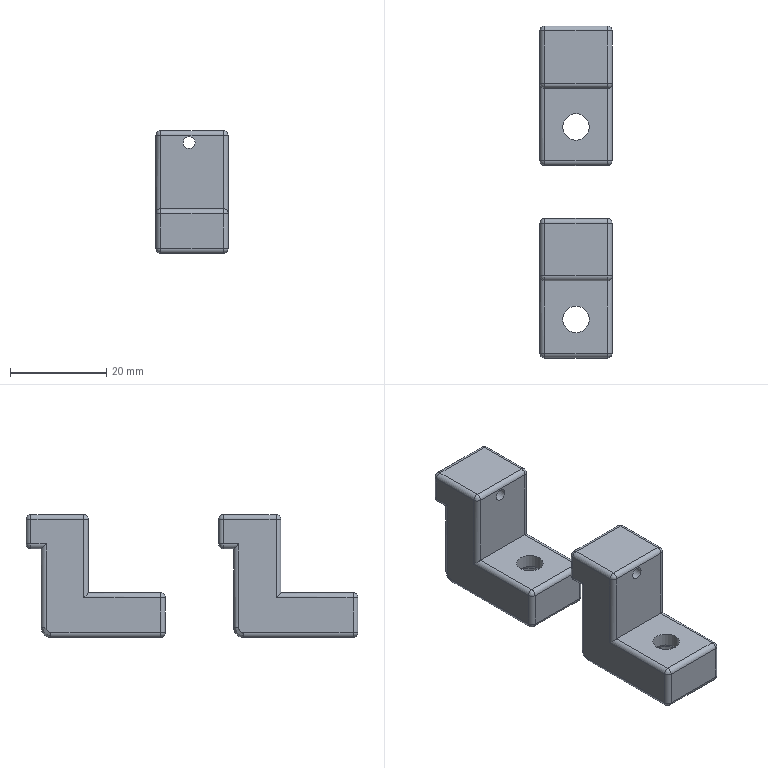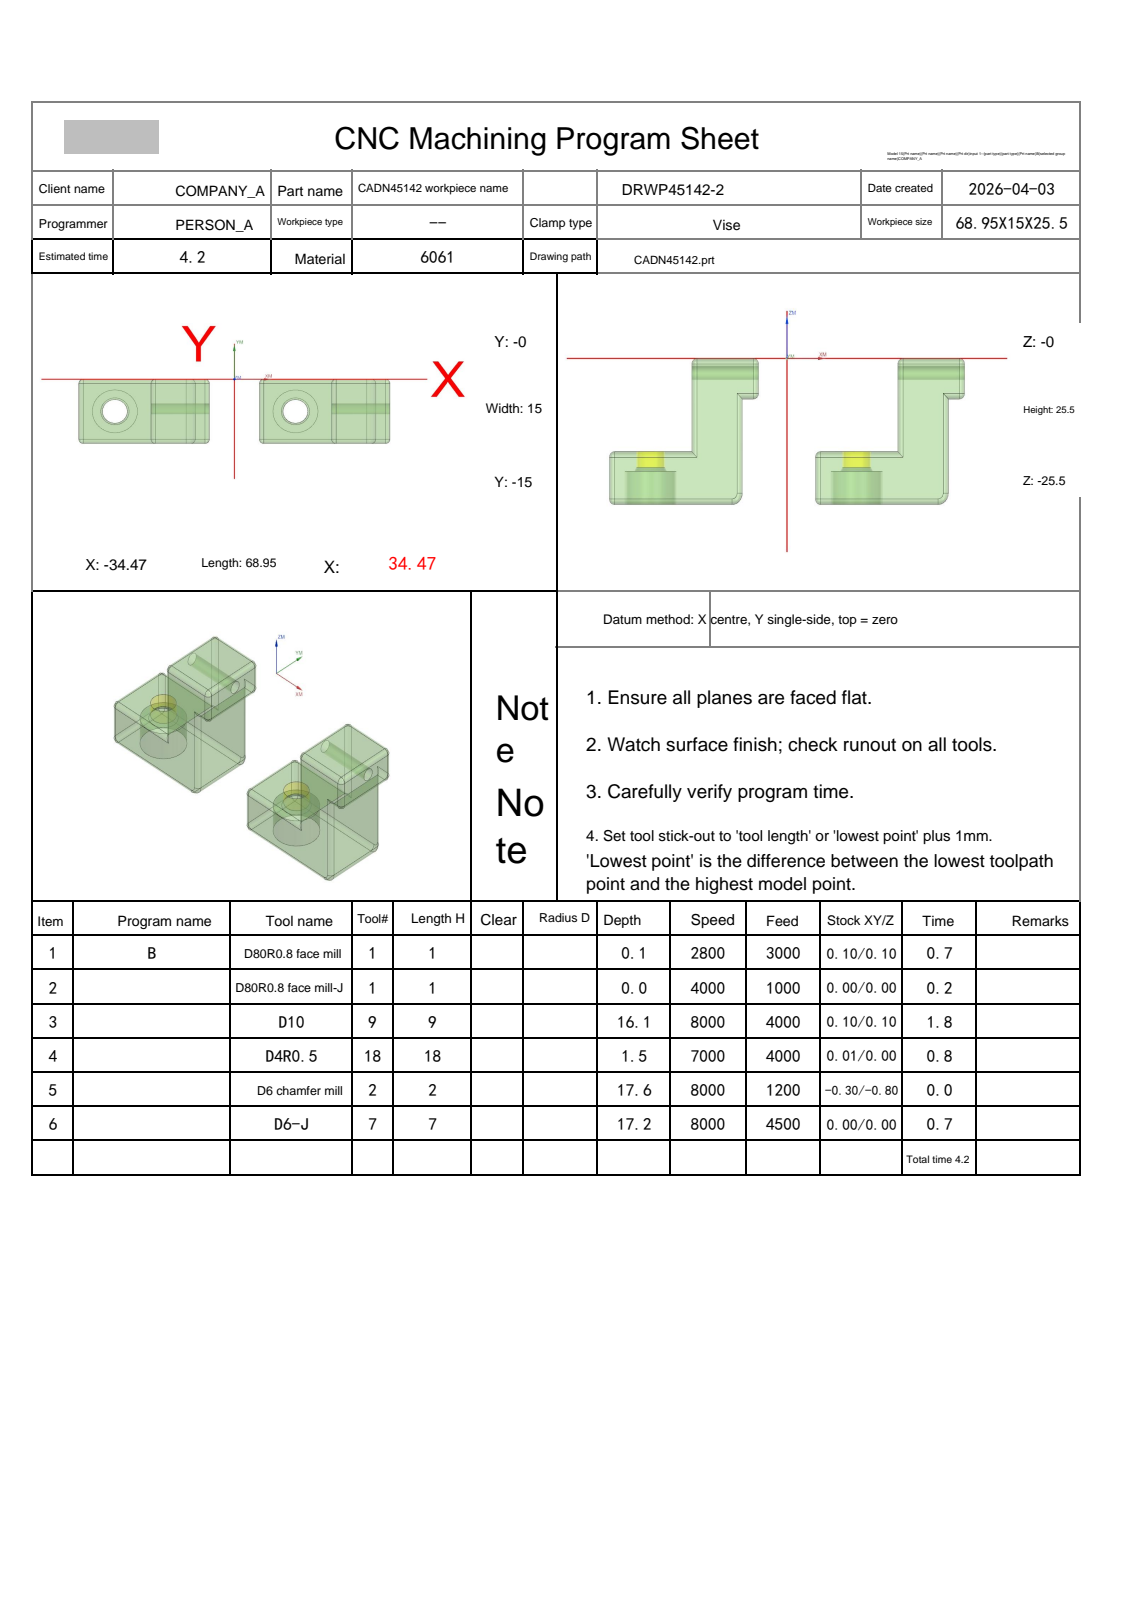NC program | NX | posted by the shop | part box 15 x 68.95 x 25.5 mm
Lines 1 to 1497 of 8513:
%
O0001
(Machine time: 5.39 MIN)
(===Total Tool:5===)
(T1=D80R0.8 face mill D=80.  R=0.8  D-  H01 Z=-0.   )
(T9=D10     D=10.  R=0.   D-  H09 Z=-16.15)
(T18=D4R0.5 D=4.   R=0.5  D-  H18 Z=-1.5  )
(T2=D6 chamfer mill   D=6.   R=0.   D-  H02 Z=-17.65)
(T7=D6-J    D=6.   R=0.   D7  H07 Z=-17.25)
G80 G90 G17 G49 G40
G91 G28 Z0
M01
N1 T01 M06
(D80R0.8 face mill D=80. R=0.8 H=01 ce=0.10 di=0.10)
G00 G90 G54 X86.572 Y-5.569 M03 S2800
G43 H01 Z20.
M08
Z6.011
G01 Z4.011 F3000.
X74.572 Y-5.836
X-74.572 Y-9.163
X-86.572 Y-9.431
Z6.011
G00 X86.572 Y-5.569
Z5.522
G01 Z3.522
X74.572 Y-5.836
X-74.572 Y-9.163
X-86.572 Y-9.431
Z5.522
G00 X86.572 Y-5.569
Z5.033
G01 Z3.033
X74.572 Y-5.836
X-74.572 Y-9.163
X-86.572 Y-9.431
Z5.033
G00 X86.572 Y-5.569
Z4.544
G01 Z2.544
X74.572 Y-5.836
X-74.572 Y-9.163
X-86.572 Y-9.431
Z4.544
G00 Z20.
X86.572 Y-5.569
Z4.056
G01 Z2.056
X74.572 Y-5.836
X-74.572 Y-9.163
X-86.572 Y-9.431
Z4.056
G00 Z20.
X86.572 Y-5.569
Z3.567
G01 Z1.567
X74.572 Y-5.836
X-74.572 Y-9.163
X-86.572 Y-9.431
Z3.567
G00 Z20.
X86.572 Y-5.569
Z3.078
G01 Z1.078
X74.572 Y-5.836
X-74.572 Y-9.163
X-86.572 Y-9.431
Z3.078
G00 Z20.
X86.572 Y-5.569
Z2.589
G01 Z.589
X74.572 Y-5.836
X-74.572 Y-9.163
X-86.572 Y-9.431
Z2.589
G00 Z20.
X86.572 Y-5.569
Z2.1
G01 Z.1
X74.572 Y-5.836
X-74.572 Y-9.163
X-86.572 Y-9.431
Z2.1
G00 Z20.
G91 G28 Z0.0
M05
M09
G91 G28 Z0.0
M01
N2 T01 M06
(D80R0.8 face mill-J  D=80. R=0.8 H=01 ce=0.00 di=0.00)
G00 G90 G54 X86.474 Y-5.572 M03 S4000
G43 H01 Z20.
M08
Z2.
G01 Z0.0 F1000.
X74.474 Y-5.84
X-74.474 Y-9.16
X-86.474 Y-9.427
Z2.
G00 Z20.
G91 G28 Z0.0
M05
M09
G91 G28 Z0.0
M01
N3 T09 M06
(D10  D=10. R=0. H=09 ce=0.10 di=0.10)
G00 G90 G54 X9.025 Y7. M03 S8000
G43 H09 Z14.
M08
Z.902
G01 Z-.598 F4000.
Y3.9
X18.892
G03 X16.425 Y-1. I3.633 J-4.9
G01 Y-14.
G03 X18.892 Y-18.9 I6.1 J0.0
G01 X1.625
Y3.9
X6.357
G02 X7.069 Y3.602 I0.0 J-1.
G01 X11.138 Y-.529
G03 X11.388 Y-.713 I.712 J.702
G02 X11.925 Y-1.599 I-.462 J-.887
G01 Y-13.401
G02 X10.927 Y-14.4 I-1. J.001
G01 X7.124
G02 X6.125 Y-13.401 I.001 J1.
G01 Y-1.599
G02 X7.124 Y-.6 I1. J-.001
G01 X9.025
X9.525
Y7.
Z.902
G00 X9.025
Z.304
G01 Z-1.196
Y3.9
X18.892
G03 X16.425 Y-1. I3.633 J-4.9
G01 Y-14.
G03 X18.892 Y-18.9 I6.1 J0.0
G01 X1.625
Y3.9
X6.357
G02 X7.069 Y3.602 I0.0 J-1.
G01 X11.138 Y-.529
G03 X11.388 Y-.713 I.712 J.702
G02 X11.925 Y-1.599 I-.462 J-.887
G01 Y-13.401
G02 X10.927 Y-14.4 I-1. J.001
G01 X7.124
G02 X6.125 Y-13.401 I.001 J1.
G01 Y-1.599
G02 X7.124 Y-.6 I1. J-.001
G01 X9.025
X9.525
Y7.
Z.304
G00 X9.025
Z-.294
G01 Z-1.794
Y3.9
X18.892
G03 X16.425 Y-1. I3.633 J-4.9
G01 Y-14.
G03 X18.892 Y-18.9 I6.1 J0.0
G01 X1.625
Y3.9
X6.357
G02 X7.069 Y3.602 I0.0 J-1.
G01 X11.138 Y-.529
G03 X11.388 Y-.713 I.712 J.702
G02 X11.925 Y-1.599 I-.462 J-.887
G01 Y-13.401
G02 X10.927 Y-14.4 I-1. J.001
G01 X7.124
G02 X6.125 Y-13.401 I.001 J1.
G01 Y-1.599
G02 X7.124 Y-.6 I1. J-.001
G01 X9.025
X9.525
Y7.
Z-.294
G00 X9.025
Z-.893
G01 Z-2.393
Y3.9
X18.892
G03 X16.425 Y-1. I3.633 J-4.9
G01 Y-14.
G03 X18.892 Y-18.9 I6.1 J0.0
G01 X1.625
Y3.9
X6.357
G02 X7.069 Y3.602 I0.0 J-1.
G01 X11.138 Y-.529
G03 X11.388 Y-.713 I.712 J.702
G02 X11.925 Y-1.599 I-.462 J-.887
G01 Y-13.401
G02 X10.927 Y-14.4 I-1. J.001
G01 X7.124
G02 X6.125 Y-13.401 I.001 J1.
G01 Y-1.599
G02 X7.124 Y-.6 I1. J-.001
G01 X9.025
X9.525
Y7.
Z-.893
G00 X9.025
Z-1.491
G01 Z-2.991
Y3.9
X18.892
G03 X16.425 Y-1. I3.633 J-4.9
G01 Y-14.
G03 X18.892 Y-18.9 I6.1 J0.0
G01 X1.625
Y3.9
X6.357
G02 X7.069 Y3.602 I0.0 J-1.
G01 X11.138 Y-.529
G03 X11.388 Y-.713 I.712 J.702
G02 X11.925 Y-1.599 I-.462 J-.887
G01 Y-13.401
G02 X10.927 Y-14.4 I-1. J.001
G01 X7.124
G02 X6.125 Y-13.401 I.001 J1.
G01 Y-1.599
G02 X7.124 Y-.6 I1. J-.001
G01 X9.025
X9.525
Y7.
Z-1.491
G00 X9.025
Z-2.089
G01 Z-3.589
Y3.9
X18.892
G03 X16.425 Y-1. I3.633 J-4.9
G01 Y-14.
G03 X18.892 Y-18.9 I6.1 J0.0
G01 X1.625
Y3.9
X6.357
G02 X7.069 Y3.602 I0.0 J-1.
G01 X11.138 Y-.529
G03 X11.388 Y-.713 I.712 J.702
G02 X11.925 Y-1.599 I-.462 J-.887
G01 Y-13.401
G02 X10.927 Y-14.4 I-1. J.001
G01 X7.124
G02 X6.125 Y-13.401 I.001 J1.
G01 Y-1.599
G02 X7.124 Y-.6 I1. J-.001
G01 X9.025
X9.525
Y7.
Z-2.089
G00 X9.025
Z-2.687
G01 Z-4.187
Y3.9
X18.892
G03 X16.425 Y-1. I3.633 J-4.9
G01 Y-14.
G03 X18.892 Y-18.9 I6.1 J0.0
G01 X1.625
Y3.9
X6.357
G02 X7.069 Y3.602 I0.0 J-1.
G01 X11.138 Y-.529
G03 X11.388 Y-.713 I.712 J.702
G02 X11.925 Y-1.599 I-.462 J-.887
G01 Y-13.401
G02 X10.927 Y-14.4 I-1. J.001
G01 X7.124
G02 X6.125 Y-13.401 I.001 J1.
G01 Y-1.599
G02 X7.124 Y-.6 I1. J-.001
G01 X9.025
X9.525
Y7.
Z-2.687
G00 X9.025
Z-3.285
G01 Z-4.785
Y3.9
X18.892
G03 X16.425 Y-1. I3.633 J-4.9
G01 Y-14.
G03 X18.892 Y-18.9 I6.1 J0.0
G01 X1.625
Y3.9
X6.357
G02 X7.069 Y3.602 I0.0 J-1.
G01 X11.138 Y-.529
G03 X11.388 Y-.713 I.712 J.702
G02 X11.925 Y-1.599 I-.462 J-.887
G01 Y-13.401
G02 X10.927 Y-14.4 I-1. J.001
G01 X7.124
G02 X6.125 Y-13.401 I.001 J1.
G01 Y-1.599
G02 X7.124 Y-.6 I1. J-.001
G01 X9.025
X9.525
Y7.
Z-3.285
G00 X9.025
Z-3.883
G01 Z-5.383
Y3.9
X18.892
G03 X16.425 Y-1. I3.633 J-4.9
G01 Y-14.
G03 X18.892 Y-18.9 I6.1 J0.0
G01 X1.625
Y3.9
X6.357
G02 X7.069 Y3.602 I0.0 J-1.
G01 X11.138 Y-.529
G03 X11.388 Y-.713 I.712 J.702
G02 X11.925 Y-1.599 I-.462 J-.887
G01 Y-13.401
G02 X10.927 Y-14.4 I-1. J.001
G01 X7.124
G02 X6.125 Y-13.401 I.001 J1.
G01 Y-1.599
G02 X7.124 Y-.6 I1. J-.001
G01 X9.025
X9.525
Y7.
Z-3.883
G00 X9.025
Z-4.481
G01 Z-5.981
Y3.9
X18.892
G03 X16.425 Y-1. I3.633 J-4.9
G01 Y-14.
G03 X18.892 Y-18.9 I6.1 J0.0
G01 X1.625
Y3.9
X6.357
G02 X7.069 Y3.602 I0.0 J-1.
G01 X11.138 Y-.529
G03 X11.388 Y-.713 I.712 J.702
G02 X11.925 Y-1.599 I-.462 J-.887
G01 Y-13.401
G02 X10.927 Y-14.4 I-1. J.001
G01 X7.124
G02 X6.125 Y-13.401 I.001 J1.
G01 Y-1.599
G02 X7.124 Y-.6 I1. J-.001
G01 X9.025
X9.525
Y7.
Z-4.481
G00 X9.025
Z-5.08
G01 Z-6.58
Y3.9
X18.892
G03 X16.425 Y-1. I3.633 J-4.9
G01 Y-14.
G03 X18.892 Y-18.9 I6.1 J0.0
G01 X1.625
Y3.9
X6.357
G02 X7.069 Y3.602 I0.0 J-1.
G01 X11.138 Y-.529
G03 X11.388 Y-.713 I.712 J.702
G02 X11.925 Y-1.599 I-.462 J-.887
G01 Y-13.401
G02 X10.927 Y-14.4 I-1. J.001
G01 X7.124
G02 X6.125 Y-13.401 I.001 J1.
G01 Y-1.599
G02 X7.124 Y-.6 I1. J-.001
G01 X9.025
X9.525
Y7.
Z-5.08
G00 X9.025
Z-5.678
G01 Z-7.178
Y3.9
X18.892
G03 X16.425 Y-1. I3.633 J-4.9
G01 Y-14.
G03 X18.892 Y-18.9 I6.1 J0.0
G01 X1.625
Y3.9
X6.357
G02 X7.069 Y3.602 I0.0 J-1.
G01 X11.138 Y-.529
G03 X11.388 Y-.713 I.712 J.702
G02 X11.925 Y-1.599 I-.462 J-.887
G01 Y-13.401
G02 X10.927 Y-14.4 I-1. J.001
G01 X7.124
G02 X6.125 Y-13.401 I.001 J1.
G01 Y-1.599
G02 X7.124 Y-.6 I1. J-.001
G01 X9.025
X9.525
Y7.
Z-5.678
G00 X9.025
Z-6.276
G01 Z-7.776
Y3.9
X18.892
G03 X16.425 Y-1. I3.633 J-4.9
G01 Y-14.
G03 X18.892 Y-18.9 I6.1 J0.0
G01 X1.625
Y3.9
X6.357
G02 X7.069 Y3.602 I0.0 J-1.
G01 X11.138 Y-.529
G03 X11.388 Y-.713 I.712 J.702
G02 X11.925 Y-1.599 I-.462 J-.887
G01 Y-13.401
G02 X10.927 Y-14.4 I-1. J.001
G01 X7.124
G02 X6.125 Y-13.401 I.001 J1.
G01 Y-1.599
G02 X7.124 Y-.6 I1. J-.001
G01 X9.025
X9.525
Y7.
Z-6.276
G00 X9.025
Z-6.874
G01 Z-8.374
Y3.9
X18.892
G03 X16.425 Y-1. I3.633 J-4.9
G01 Y-14.
G03 X18.892 Y-18.9 I6.1 J0.0
G01 X1.625
Y3.9
X6.357
G02 X7.069 Y3.602 I0.0 J-1.
G01 X11.138 Y-.529
G03 X11.388 Y-.713 I.712 J.702
G02 X11.925 Y-1.599 I-.462 J-.887
G01 Y-13.401
G02 X10.927 Y-14.4 I-1. J.001
G01 X7.124
G02 X6.125 Y-13.401 I.001 J1.
G01 Y-1.599
G02 X7.124 Y-.6 I1. J-.001
G01 X9.025
X9.525
Y7.
Z-6.874
G00 X9.025
Z-7.472
G01 Z-8.972
Y3.9
X18.892
G03 X16.425 Y-1. I3.633 J-4.9
G01 Y-14.
G03 X18.892 Y-18.9 I6.1 J0.0
G01 X1.625
Y3.9
X6.357
G02 X7.069 Y3.602 I0.0 J-1.
G01 X11.138 Y-.529
G03 X11.388 Y-.713 I.712 J.702
G02 X11.925 Y-1.599 I-.462 J-.887
G01 Y-13.401
G02 X10.927 Y-14.4 I-1. J.001
G01 X7.124
G02 X6.125 Y-13.401 I.001 J1.
G01 Y-1.599
G02 X7.124 Y-.6 I1. J-.001
G01 X9.025
X9.525
Y7.
Z-7.472
G00 X9.025
Z-8.07
G01 Z-9.57
Y3.9
X18.892
G03 X16.425 Y-1. I3.633 J-4.9
G01 Y-14.
G03 X18.892 Y-18.9 I6.1 J0.0
G01 X1.625
Y3.9
X6.357
G02 X7.069 Y3.602 I0.0 J-1.
G01 X11.138 Y-.529
G03 X11.388 Y-.713 I.712 J.702
G02 X11.925 Y-1.599 I-.462 J-.887
G01 Y-13.401
G02 X10.927 Y-14.4 I-1. J.001
G01 X7.124
G02 X6.125 Y-13.401 I.001 J1.
G01 Y-1.599
G02 X7.124 Y-.6 I1. J-.001
G01 X9.025
X9.525
Y7.
Z-8.07
G00 X9.025
Z-8.669
G01 Z-10.169
Y3.9
X18.892
G03 X16.425 Y-1. I3.633 J-4.9
G01 Y-14.
G03 X18.892 Y-18.9 I6.1 J0.0
G01 X1.625
Y3.9
X6.357
G02 X7.069 Y3.602 I0.0 J-1.
G01 X11.138 Y-.529
G03 X11.388 Y-.713 I.712 J.702
G02 X11.925 Y-1.599 I-.462 J-.887
G01 Y-13.401
G02 X10.927 Y-14.4 I-1. J.001
G01 X7.124
G02 X6.125 Y-13.401 I.001 J1.
G01 Y-1.599
G02 X7.124 Y-.6 I1. J-.001
G01 X9.025
X9.525
Y7.
Z-8.669
G00 X9.025
Z-9.267
G01 Z-10.767
Y3.9
X18.892
G03 X16.425 Y-1. I3.633 J-4.9
G01 Y-14.
G03 X18.892 Y-18.9 I6.1 J0.0
G01 X1.625
Y3.9
X6.357
G02 X7.069 Y3.602 I0.0 J-1.
G01 X11.138 Y-.529
G03 X11.388 Y-.713 I.712 J.702
G02 X11.925 Y-1.599 I-.462 J-.887
G01 Y-13.401
G02 X10.927 Y-14.4 I-1. J.001
G01 X7.124
G02 X6.125 Y-13.401 I.001 J1.
G01 Y-1.599
G02 X7.124 Y-.6 I1. J-.001
G01 X9.025
X9.525
Y7.
Z-9.267
G00 X9.025
Z-9.865
G01 Z-11.365
Y3.9
X18.892
G03 X16.425 Y-1. I3.633 J-4.9
G01 Y-14.
G03 X18.892 Y-18.9 I6.1 J0.0
G01 X1.625
Y3.9
X6.357
G02 X7.069 Y3.602 I0.0 J-1.
G01 X11.138 Y-.529
G03 X11.388 Y-.713 I.712 J.702
G02 X11.925 Y-1.599 I-.462 J-.887
G01 Y-13.401
G02 X10.927 Y-14.4 I-1. J.001
G01 X7.124
G02 X6.125 Y-13.401 I.001 J1.
G01 Y-1.599
G02 X7.124 Y-.6 I1. J-.001
G01 X9.025
X9.525
Y7.
Z-9.865
G00 X9.025
Z-10.463
G01 Z-11.963
Y3.9
X18.892
G03 X16.425 Y-1. I3.633 J-4.9
G01 Y-14.
G03 X18.892 Y-18.9 I6.1 J0.0
G01 X1.625
Y3.9
X6.357
G02 X7.069 Y3.602 I0.0 J-1.
G01 X11.138 Y-.529
G03 X11.388 Y-.713 I.712 J.702
G02 X11.925 Y-1.599 I-.462 J-.887
G01 Y-13.401
G02 X10.927 Y-14.4 I-1. J.001
G01 X7.124
G02 X6.125 Y-13.401 I.001 J1.
G01 Y-1.599
G02 X7.124 Y-.6 I1. J-.001
G01 X9.025
X9.525
Y7.
Z-10.463
G00 X9.025
Z-11.061
G01 Z-12.561
Y3.9
X18.892
G03 X16.425 Y-1. I3.633 J-4.9
G01 Y-14.
G03 X18.892 Y-18.9 I6.1 J0.0
G01 X1.625
Y3.9
X6.357
G02 X7.069 Y3.602 I0.0 J-1.
G01 X11.138 Y-.529
G03 X11.388 Y-.713 I.712 J.702
G02 X11.925 Y-1.599 I-.462 J-.887
G01 Y-13.401
G02 X10.927 Y-14.4 I-1. J.001
G01 X7.124
G02 X6.125 Y-13.401 I.001 J1.
G01 Y-1.599
G02 X7.124 Y-.6 I1. J-.001
G01 X9.025
X9.525
Y7.
Z-11.061
G00 X9.025
Z-11.659
G01 Z-13.159
Y3.9
X18.892
G03 X16.425 Y-1. I3.633 J-4.9
G01 Y-14.
G03 X18.892 Y-18.9 I6.1 J0.0
G01 X1.625
Y3.9
X6.357
G02 X7.069 Y3.602 I0.0 J-1.
G01 X11.138 Y-.529
G03 X11.388 Y-.713 I.712 J.702
G02 X11.925 Y-1.599 I-.462 J-.887
G01 Y-13.401
G02 X10.927 Y-14.4 I-1. J.001
G01 X7.124
G02 X6.125 Y-13.401 I.001 J1.
G01 Y-1.599
G02 X7.124 Y-.6 I1. J-.001
G01 X9.025
X9.525
Y7.
Z-11.659
G00 X9.025
Z-12.257
G01 Z-13.757
Y3.9
X18.892
G03 X16.425 Y-1. I3.633 J-4.9
G01 Y-14.
G03 X18.892 Y-18.9 I6.1 J0.0
G01 X1.625
Y3.9
X6.357
G02 X7.069 Y3.602 I0.0 J-1.
G01 X11.138 Y-.529
G03 X11.388 Y-.713 I.712 J.702
G02 X11.925 Y-1.599 I-.462 J-.887
G01 Y-13.401
G02 X10.927 Y-14.4 I-1. J.001
G01 X7.124
G02 X6.125 Y-13.401 I.001 J1.
G01 Y-1.599
G02 X7.124 Y-.6 I1. J-.001
G01 X9.025
X9.525
Y7.
Z-12.257
G00 X9.025
Z-12.856
G01 Z-14.356
Y3.9
X18.892
G03 X16.425 Y-1. I3.633 J-4.9
G01 Y-14.
G03 X18.892 Y-18.9 I6.1 J0.0
G01 X1.625
Y3.9
X6.357
G02 X7.069 Y3.602 I0.0 J-1.
G01 X11.138 Y-.529
G03 X11.388 Y-.713 I.712 J.702
G02 X11.925 Y-1.599 I-.462 J-.887
G01 Y-13.401
G02 X10.927 Y-14.4 I-1. J.001
G01 X7.124
G02 X6.125 Y-13.401 I.001 J1.
G01 Y-1.599
G02 X7.124 Y-.6 I1. J-.001
G01 X9.025
X9.525
Y7.
Z-12.856
G00 X9.025
Z-13.454
G01 Z-14.954
Y3.9
X18.892
G03 X16.425 Y-1. I3.633 J-4.9
G01 Y-14.
G03 X18.892 Y-18.9 I6.1 J0.0
G01 X1.625
Y3.9
X6.357
G02 X7.069 Y3.602 I0.0 J-1.
G01 X11.138 Y-.529
G03 X11.388 Y-.713 I.712 J.702
G02 X11.925 Y-1.599 I-.462 J-.887
G01 Y-13.401
G02 X10.927 Y-14.4 I-1. J.001
G01 X7.124
G02 X6.125 Y-13.401 I.001 J1.
G01 Y-1.599
G02 X7.124 Y-.6 I1. J-.001
G01 X9.025
X9.525
Y7.
Z-13.454
G00 X9.025
Z-14.052
G01 Z-15.552
Y3.9
X18.892
G03 X16.425 Y-1. I3.633 J-4.9
G01 Y-14.
G03 X18.892 Y-18.9 I6.1 J0.0
G01 X1.625
Y3.9
X6.357
G02 X7.069 Y3.602 I0.0 J-1.
G01 X11.138 Y-.529
G03 X11.388 Y-.713 I.712 J.702
G02 X11.925 Y-1.599 I-.462 J-.887
G01 Y-13.401
G02 X10.927 Y-14.4 I-1. J.001
G01 X7.124
G02 X6.125 Y-13.401 I.001 J1.
G01 Y-1.599
G02 X7.124 Y-.6 I1. J-.001
G01 X9.025
X9.525
Y7.
Z-14.052
G00 X9.025
Z-14.65
G01 Z-16.15
Y3.9
X18.892
G03 X16.425 Y-1. I3.633 J-4.9
G01 Y-14.
G03 X18.892 Y-18.9 I6.1 J0.0
G01 X1.625
Y3.9
X6.357
G02 X7.069 Y3.602 I0.0 J-1.
G01 X11.138 Y-.529
G03 X11.388 Y-.713 I.712 J.702
G02 X11.925 Y-1.599 I-.462 J-.887
G01 Y-13.401
G02 X10.927 Y-14.4 I-1. J.001
G01 X7.124
G02 X6.125 Y-13.401 I.001 J1.
G01 Y-1.599
G02 X7.124 Y-.6 I1. J-.001
G01 X9.025
X9.525
Y7.
Z-14.65
G00 Z14.
X-41.475 Y-7.5
Z.902
G01 Z-.598
X-38.375
Y3.9
X-21.108
G03 X-23.575 Y-1. I3.633 J-4.9
G01 Y-14.
G03 X-21.108 Y-18.9 I6.1 J0.0
G01 X-38.375
Y-10.164
G02 X-38.082 Y-9.457 I1. J0.0
G01 X-34.167 Y-5.543
G03 X-33.875 Y-4.836 I-.707 J.707
G01 Y-1.599
G02 X-32.876 Y-.6 I1. J-.001
G01 X-29.074
G02 X-28.075 Y-1.599 I-.001 J-1.
G01 Y-13.401
G02 X-29.074 Y-14.4 I-1. J.001
G01 X-32.876
G02 X-33.875 Y-13.401 I.001 J1.
G01 Y-7.5
Y-7.
X-41.475
Z.902
G00 Y-7.5
Z.304
G01 Z-1.196
X-38.375
Y3.9
X-21.108
G03 X-23.575 Y-1. I3.633 J-4.9
G01 Y-14.
G03 X-21.108 Y-18.9 I6.1 J0.0
G01 X-38.375
Y-10.164
G02 X-38.082 Y-9.457 I1. J0.0
G01 X-34.167 Y-5.543
G03 X-33.875 Y-4.836 I-.707 J.707
G01 Y-1.599
G02 X-32.876 Y-.6 I1. J-.001
G01 X-29.074
G02 X-28.075 Y-1.599 I-.001 J-1.
G01 Y-13.401
G02 X-29.074 Y-14.4 I-1. J.001
G01 X-32.876
G02 X-33.875 Y-13.401 I.001 J1.
G01 Y-7.5
Y-7.
X-41.475
Z.304
G00 Y-7.5
Z-.294
G01 Z-1.794
X-38.375
Y3.9
X-21.108
G03 X-23.575 Y-1. I3.633 J-4.9
G01 Y-14.
G03 X-21.108 Y-18.9 I6.1 J0.0
G01 X-38.375
Y-10.164
G02 X-38.082 Y-9.457 I1. J0.0
G01 X-34.167 Y-5.543
G03 X-33.875 Y-4.836 I-.707 J.707
G01 Y-1.599
G02 X-32.876 Y-.6 I1. J-.001
G01 X-29.074
G02 X-28.075 Y-1.599 I-.001 J-1.
G01 Y-13.401
G02 X-29.074 Y-14.4 I-1. J.001
G01 X-32.876
G02 X-33.875 Y-13.401 I.001 J1.
G01 Y-7.5
Y-7.
X-41.475
Z-.294
G00 Y-7.5
Z-.893
G01 Z-2.393
X-38.375
Y3.9
X-21.108
G03 X-23.575 Y-1. I3.633 J-4.9
G01 Y-14.
G03 X-21.108 Y-18.9 I6.1 J0.0
G01 X-38.375
Y-10.164
G02 X-38.082 Y-9.457 I1. J0.0
G01 X-34.167 Y-5.543
G03 X-33.875 Y-4.836 I-.707 J.707
G01 Y-1.599
G02 X-32.876 Y-.6 I1. J-.001
G01 X-29.074
G02 X-28.075 Y-1.599 I-.001 J-1.
G01 Y-13.401
G02 X-29.074 Y-14.4 I-1. J.001
G01 X-32.876
G02 X-33.875 Y-13.401 I.001 J1.
G01 Y-7.5
Y-7.
X-41.475
Z-.893
G00 Y-7.5
Z-1.491
G01 Z-2.991
X-38.375
Y3.9
X-21.108
G03 X-23.575 Y-1. I3.633 J-4.9
G01 Y-14.
G03 X-21.108 Y-18.9 I6.1 J0.0
G01 X-38.375
Y-10.164
G02 X-38.082 Y-9.457 I1. J0.0
G01 X-34.167 Y-5.543
G03 X-33.875 Y-4.836 I-.707 J.707
G01 Y-1.599
G02 X-32.876 Y-.6 I1. J-.001
G01 X-29.074
G02 X-28.075 Y-1.599 I-.001 J-1.
G01 Y-13.401
G02 X-29.074 Y-14.4 I-1. J.001
G01 X-32.876
G02 X-33.875 Y-13.401 I.001 J1.
G01 Y-7.5
Y-7.
X-41.475
Z-1.491
G00 Y-7.5
Z-2.089
G01 Z-3.589
X-38.375
Y3.9
X-21.108
G03 X-23.575 Y-1. I3.633 J-4.9
G01 Y-14.
G03 X-21.108 Y-18.9 I6.1 J0.0
G01 X-38.375
Y-10.164
G02 X-38.082 Y-9.457 I1. J0.0
G01 X-34.167 Y-5.543
G03 X-33.875 Y-4.836 I-.707 J.707
G01 Y-1.599
G02 X-32.876 Y-.6 I1. J-.001
G01 X-29.074
G02 X-28.075 Y-1.599 I-.001 J-1.
G01 Y-13.401
G02 X-29.074 Y-14.4 I-1. J.001
G01 X-32.876
G02 X-33.875 Y-13.401 I.001 J1.
G01 Y-7.5
Y-7.
X-41.475
Z-2.089
G00 Y-7.5
Z-2.687
G01 Z-4.187
X-38.375
Y3.9
X-21.108
G03 X-23.575 Y-1. I3.633 J-4.9
G01 Y-14.
G03 X-21.108 Y-18.9 I6.1 J0.0
G01 X-38.375
Y-10.164
G02 X-38.082 Y-9.457 I1. J0.0
G01 X-34.167 Y-5.543
G03 X-33.875 Y-4.836 I-.707 J.707
G01 Y-1.599
G02 X-32.876 Y-.6 I1. J-.001
G01 X-29.074
G02 X-28.075 Y-1.599 I-.001 J-1.
G01 Y-13.401
G02 X-29.074 Y-14.4 I-1. J.001
G01 X-32.876
G02 X-33.875 Y-13.401 I.001 J1.
G01 Y-7.5
Y-7.
X-41.475
Z-2.687
G00 Y-7.5
Z-3.285
G01 Z-4.785
X-38.375
Y3.9
X-21.108
G03 X-23.575 Y-1. I3.633 J-4.9
G01 Y-14.
G03 X-21.108 Y-18.9 I6.1 J0.0
G01 X-38.375
Y-10.164
G02 X-38.082 Y-9.457 I1. J0.0
G01 X-34.167 Y-5.543
G03 X-33.875 Y-4.836 I-.707 J.707
G01 Y-1.599
G02 X-32.876 Y-.6 I1. J-.001
G01 X-29.074
G02 X-28.075 Y-1.599 I-.001 J-1.
G01 Y-13.401
G02 X-29.074 Y-14.4 I-1. J.001
G01 X-32.876
G02 X-33.875 Y-13.401 I.001 J1.
G01 Y-7.5
Y-7.
X-41.475
Z-3.285
G00 Y-7.5
Z-3.883
G01 Z-5.383
X-38.375
Y3.9
X-21.108
G03 X-23.575 Y-1. I3.633 J-4.9
G01 Y-14.
G03 X-21.108 Y-18.9 I6.1 J0.0
G01 X-38.375
Y-10.164
G02 X-38.082 Y-9.457 I1. J0.0
G01 X-34.167 Y-5.543
G03 X-33.875 Y-4.836 I-.707 J.707
G01 Y-1.599
G02 X-32.876 Y-.6 I1. J-.001
G01 X-29.074
G02 X-28.075 Y-1.599 I-.001 J-1.
G01 Y-13.401
G02 X-29.074 Y-14.4 I-1. J.001
G01 X-32.876
G02 X-33.875 Y-13.401 I.001 J1.
G01 Y-7.5
Y-7.
X-41.475
Z-3.883
G00 Y-7.5
Z-4.481
G01 Z-5.981
X-38.375
Y3.9
X-21.108
G03 X-23.575 Y-1. I3.633 J-4.9
G01 Y-14.
G03 X-21.108 Y-18.9 I6.1 J0.0
G01 X-38.375
Y-10.164
G02 X-38.082 Y-9.457 I1. J0.0
G01 X-34.167 Y-5.543
G03 X-33.875 Y-4.836 I-.707 J.707
G01 Y-1.599
G02 X-32.876 Y-.6 I1. J-.001
G01 X-29.074
G02 X-28.075 Y-1.599 I-.001 J-1.
G01 Y-13.401
G02 X-29.074 Y-14.4 I-1. J.001
G01 X-32.876
G02 X-33.875 Y-13.401 I.001 J1.
G01 Y-7.5
Y-7.
X-41.475
Z-4.481
G00 Y-7.5
Z-5.08
G01 Z-6.58
X-38.375
Y3.9
X-21.108
G03 X-23.575 Y-1. I3.633 J-4.9
G01 Y-14.
G03 X-21.108 Y-18.9 I6.1 J0.0
G01 X-38.375
Y-10.164
G02 X-38.082 Y-9.457 I1. J0.0
G01 X-34.167 Y-5.543
G03 X-33.875 Y-4.836 I-.707 J.707
G01 Y-1.599
G02 X-32.876 Y-.6 I1. J-.001
G01 X-29.074
G02 X-28.075 Y-1.599 I-.001 J-1.
G01 Y-13.401
G02 X-29.074 Y-14.4 I-1. J.001
G01 X-32.876
G02 X-33.875 Y-13.401 I.001 J1.
G01 Y-7.5
Y-7.
X-41.475
Z-5.08
G00 Y-7.5
Z-5.678
G01 Z-7.178
X-38.375
Y3.9
X-21.108
G03 X-23.575 Y-1. I3.633 J-4.9
G01 Y-14.
G03 X-21.108 Y-18.9 I6.1 J0.0
G01 X-38.375
Y-10.164
G02 X-38.082 Y-9.457 I1. J0.0
G01 X-34.167 Y-5.543
G03 X-33.875 Y-4.836 I-.707 J.707
G01 Y-1.599
G02 X-32.876 Y-.6 I1. J-.001
G01 X-29.074
G02 X-28.075 Y-1.599 I-.001 J-1.
G01 Y-13.401
G02 X-29.074 Y-14.4 I-1. J.001
G01 X-32.876
G02 X-33.875 Y-13.401 I.001 J1.
G01 Y-7.5
Y-7.
X-41.475
Z-5.678
G00 Y-7.5
Z-6.276
G01 Z-7.776
X-38.375
Y3.9
X-21.108
G03 X-23.575 Y-1. I3.633 J-4.9
G01 Y-14.
G03 X-21.108 Y-18.9 I6.1 J0.0
G01 X-38.375
Y-10.164
G02 X-38.082 Y-9.457 I1. J0.0
G01 X-34.167 Y-5.543
G03 X-33.875 Y-4.836 I-.707 J.707
G01 Y-1.599
G02 X-32.876 Y-.6 I1. J-.001
G01 X-29.074
G02 X-28.075 Y-1.599 I-.001 J-1.
G01 Y-13.401
G02 X-29.074 Y-14.4 I-1. J.001
G01 X-32.876
G02 X-33.875 Y-13.401 I.001 J1.
G01 Y-7.5
Y-7.
X-41.475
Z-6.276
G00 Y-7.5
Z-6.874
G01 Z-8.374
X-38.375
Y3.9
X-21.108
G03 X-23.575 Y-1. I3.633 J-4.9
G01 Y-14.
G03 X-21.108 Y-18.9 I6.1 J0.0
G01 X-38.375
Y-10.164
G02 X-38.082 Y-9.457 I1. J0.0
G01 X-34.167 Y-5.543
G03 X-33.875 Y-4.836 I-.707 J.707
G01 Y-1.599
G02 X-32.876 Y-.6 I1. J-.001
G01 X-29.074
G02 X-28.075 Y-1.599 I-.001 J-1.
G01 Y-13.401
G02 X-29.074 Y-14.4 I-1. J.001
G01 X-32.876
G02 X-33.875 Y-13.401 I.001 J1.
G01 Y-7.5
Y-7.
X-41.475
Z-6.874
G00 Y-7.5
Z-7.472
G01 Z-8.972
X-38.375
Y3.9
X-21.108
G03 X-23.575 Y-1. I3.633 J-4.9
G01 Y-14.
G03 X-21.108 Y-18.9 I6.1 J0.0
G01 X-38.375
Y-10.164
G02 X-38.082 Y-9.457 I1. J0.0
G01 X-34.167 Y-5.543
G03 X-33.875 Y-4.836 I-.707 J.707
G01 Y-1.599
G02 X-32.876 Y-.6 I1. J-.001
G01 X-29.074
G02 X-28.075 Y-1.599 I-.001 J-1.
G01 Y-13.401
G02 X-29.074 Y-14.4 I-1. J.001
G01 X-32.876
G02 X-33.875 Y-13.401 I.001 J1.
G01 Y-7.5
Y-7.
X-41.475
Z-7.472
G00 Y-7.5
Z-8.07
G01 Z-9.57
X-38.375
Y3.9
X-21.108
G03 X-23.575 Y-1. I3.633 J-4.9
G01 Y-14.
G03 X-21.108 Y-18.9 I6.1 J0.0
G01 X-38.375
Y-10.164
G02 X-38.082 Y-9.457 I1. J0.0
G01 X-34.167 Y-5.543
G03 X-33.875 Y-4.836 I-.707 J.707
G01 Y-1.599
G02 X-32.876 Y-.6 I1. J-.001
G01 X-29.074
G02 X-28.075 Y-1.599 I-.001 J-1.
G01 Y-13.401
G02 X-29.074 Y-14.4 I-1. J.001
G01 X-32.876
G02 X-33.875 Y-13.401 I.001 J1.
G01 Y-7.5
Y-7.
X-41.475
Z-8.07
G00 Y-7.5
Z-8.669
G01 Z-10.169
X-38.375
Y3.9
X-21.108
G03 X-23.575 Y-1. I3.633 J-4.9
G01 Y-14.
G03 X-21.108 Y-18.9 I6.1 J0.0
G01 X-38.375
Y-10.164
G02 X-38.082 Y-9.457 I1. J0.0
G01 X-34.167 Y-5.543
G03 X-33.875 Y-4.836 I-.707 J.707
G01 Y-1.599
G02 X-32.876 Y-.6 I1. J-.001
G01 X-29.074
G02 X-28.075 Y-1.599 I-.001 J-1.
G01 Y-13.401
G02 X-29.074 Y-14.4 I-1. J.001
G01 X-32.876
G02 X-33.875 Y-13.401 I.001 J1.
G01 Y-7.5
Y-7.
X-41.475
Z-8.669
G00 Y-7.5
Z-9.267
G01 Z-10.767
X-38.375
Y3.9
X-21.108
G03 X-23.575 Y-1. I3.633 J-4.9
G01 Y-14.
G03 X-21.108 Y-18.9 I6.1 J0.0
G01 X-38.375
Y-10.164
G02 X-38.082 Y-9.457 I1. J0.0
G01 X-34.167 Y-5.543
G03 X-33.875 Y-4.836 I-.707 J.707
G01 Y-1.599
G02 X-32.876 Y-.6 I1. J-.001
G01 X-29.074
G02 X-28.075 Y-1.599 I-.001 J-1.
G01 Y-13.401
G02 X-29.074 Y-14.4 I-1. J.001
G01 X-32.876
G02 X-33.875 Y-13.401 I.001 J1.
G01 Y-7.5
Y-7.
X-41.475
Z-9.267
G00 Y-7.5
Z-9.865
G01 Z-11.365
X-38.375
Y3.9
X-21.108
G03 X-23.575 Y-1. I3.633 J-4.9
G01 Y-14.
G03 X-21.108 Y-18.9 I6.1 J0.0
G01 X-38.375
Y-10.164
G02 X-38.082 Y-9.457 I1. J0.0
G01 X-34.167 Y-5.543
G03 X-33.875 Y-4.836 I-.707 J.707
G01 Y-1.599
G02 X-32.876 Y-.6 I1. J-.001
G01 X-29.074
G02 X-28.075 Y-1.599 I-.001 J-1.
G01 Y-13.401
G02 X-29.074 Y-14.4 I-1. J.001
G01 X-32.876
G02 X-33.875 Y-13.401 I.001 J1.
G01 Y-7.5
Y-7.
X-41.475
Z-9.865
G00 Y-7.5
Z-10.463
G01 Z-11.963
X-38.375
Y3.9
X-21.108
G03 X-23.575 Y-1. I3.633 J-4.9
G01 Y-14.
G03 X-21.108 Y-18.9 I6.1 J0.0
G01 X-38.375
Y-10.164
G02 X-38.082 Y-9.457 I1. J0.0
G01 X-34.167 Y-5.543
G03 X-33.875 Y-4.836 I-.707 J.707
G01 Y-1.599
G02 X-32.876 Y-.6 I1. J-.001
G01 X-29.074
G02 X-28.075 Y-1.599 I-.001 J-1.
G01 Y-13.401
G02 X-29.074 Y-14.4 I-1. J.001
G01 X-32.876
G02 X-33.875 Y-13.401 I.001 J1.
G01 Y-7.5
Y-7.
X-41.475
Z-10.463
G00 Y-7.5
Z-11.061
G01 Z-12.561
X-38.375
Y3.9
X-21.108
G03 X-23.575 Y-1. I3.633 J-4.9
G01 Y-14.
G03 X-21.108 Y-18.9 I6.1 J0.0
G01 X-38.375
Y-10.164
G02 X-38.082 Y-9.457 I1. J0.0
G01 X-34.167 Y-5.543
G03 X-33.875 Y-4.836 I-.707 J.707
G01 Y-1.599
G02 X-32.876 Y-.6 I1. J-.001
G01 X-29.074
G02 X-28.075 Y-1.599 I-.001 J-1.
G01 Y-13.401
G02 X-29.074 Y-14.4 I-1. J.001
G01 X-32.876
G02 X-33.875 Y-13.401 I.001 J1.
G01 Y-7.5
Y-7.
X-41.475
Z-11.061
G00 Y-7.5
Z-11.659
G01 Z-13.159
X-38.375
Y3.9
X-21.108
G03 X-23.575 Y-1. I3.633 J-4.9
G01 Y-14.
G03 X-21.108 Y-18.9 I6.1 J0.0
G01 X-38.375
Y-10.164
G02 X-38.082 Y-9.457 I1. J0.0
G01 X-34.167 Y-5.543
G03 X-33.875 Y-4.836 I-.707 J.707
G01 Y-1.599
G02 X-32.876 Y-.6 I1. J-.001
G01 X-29.074
G02 X-28.075 Y-1.599 I-.001 J-1.
G01 Y-13.401
G02 X-29.074 Y-14.4 I-1. J.001
G01 X-32.876
G02 X-33.875 Y-13.401 I.001 J1.
G01 Y-7.5
Y-7.
X-41.475
Z-11.659
G00 Y-7.5
Z-12.257
G01 Z-13.757
X-38.375
Y3.9
X-21.108
G03 X-23.575 Y-1. I3.633 J-4.9
G01 Y-14.
G03 X-21.108 Y-18.9 I6.1 J0.0
G01 X-38.375
Y-10.164
G02 X-38.082 Y-9.457 I1. J0.0
G01 X-34.167 Y-5.543
G03 X-33.875 Y-4.836 I-.707 J.707
G01 Y-1.599
G02 X-32.876 Y-.6 I1. J-.001
G01 X-29.074
G02 X-28.075 Y-1.599 I-.001 J-1.
G01 Y-13.401
G02 X-29.074 Y-14.4 I-1. J.001
G01 X-32.876
G02 X-33.875 Y-13.401 I.001 J1.
G01 Y-7.5
Y-7.
X-41.475
Z-12.257
G00 Y-7.5
Z-12.856
G01 Z-14.356
X-38.375
Y3.9
X-21.108
G03 X-23.575 Y-1. I3.633 J-4.9
G01 Y-14.
G03 X-21.108 Y-18.9 I6.1 J0.0
G01 X-38.375
Y-10.164
G02 X-38.082 Y-9.457 I1. J0.0
G01 X-34.167 Y-5.543
G03 X-33.875 Y-4.836 I-.707 J.707
G01 Y-1.599
G02 X-32.876 Y-.6 I1. J-.001
G01 X-29.074
G02 X-28.075 Y-1.599 I-.001 J-1.
G01 Y-13.401
G02 X-29.074 Y-14.4 I-1. J.001
G01 X-32.876
G02 X-33.875 Y-13.401 I.001 J1.
G01 Y-7.5
Y-7.
X-41.475
Z-12.856
G00 Y-7.5
Z-13.454
G01 Z-14.954
X-38.375
Y3.9
X-21.108
G03 X-23.575 Y-1. I3.633 J-4.9
G01 Y-14.
G03 X-21.108 Y-18.9 I6.1 J0.0
G01 X-38.375
Y-10.164
G02 X-38.082 Y-9.457 I1. J0.0
G01 X-34.167 Y-5.543
G03 X-33.875 Y-4.836 I-.707 J.707
G01 Y-1.599
G02 X-32.876 Y-.6 I1. J-.001
G01 X-29.074
G02 X-28.075 Y-1.599 I-.001 J-1.
G01 Y-13.401
G02 X-29.074 Y-14.4 I-1. J.001
G01 X-32.876
G02 X-33.875 Y-13.401 I.001 J1.
G01 Y-7.5
Y-7.
X-41.475
Z-13.454
G00 Y-7.5
Z-14.052
G01 Z-15.552
X-38.375
Y3.9
X-21.108
G03 X-23.575 Y-1. I3.633 J-4.9
G01 Y-14.
G03 X-21.108 Y-18.9 I6.1 J0.0
G01 X-38.375
Y-10.164
G02 X-38.082 Y-9.457 I1. J0.0
G01 X-34.167 Y-5.543
G03 X-33.875 Y-4.836 I-.707 J.707
G01 Y-1.599
G02 X-32.876 Y-.6 I1. J-.001
G01 X-29.074
G02 X-28.075 Y-1.599 I-.001 J-1.
G01 Y-13.401
G02 X-29.074 Y-14.4 I-1. J.001
G01 X-32.876
G02 X-33.875 Y-13.401 I.001 J1.
G01 Y-7.5
Y-7.
X-41.475
Z-14.052
G00 Y-7.5
Z-14.65
G01 Z-16.15
X-38.375
Y3.9
X-21.108
G03 X-23.575 Y-1. I3.633 J-4.9
G01 Y-14.
G03 X-21.108 Y-18.9 I6.1 J0.0
G01 X-38.375
Y-10.164
G02 X-38.082 Y-9.457 I1. J0.0
G01 X-34.167 Y-5.543
G03 X-33.875 Y-4.836 I-.707 J.707
G01 Y-1.599
G02 X-32.876 Y-.6 I1. J-.001
G01 X-29.074
G02 X-28.075 Y-1.599 I-.001 J-1.
G01 Y-13.401
G02 X-29.074 Y-14.4 I-1. J.001
G01 X-32.876
G02 X-33.875 Y-13.401 I.001 J1.
G01 Y-7.5
Y-7.
X-41.475
Z-14.65
G00 Z14.
G91 G28 Z0.0
M05
M09
G91 G28 Z0.0
M01